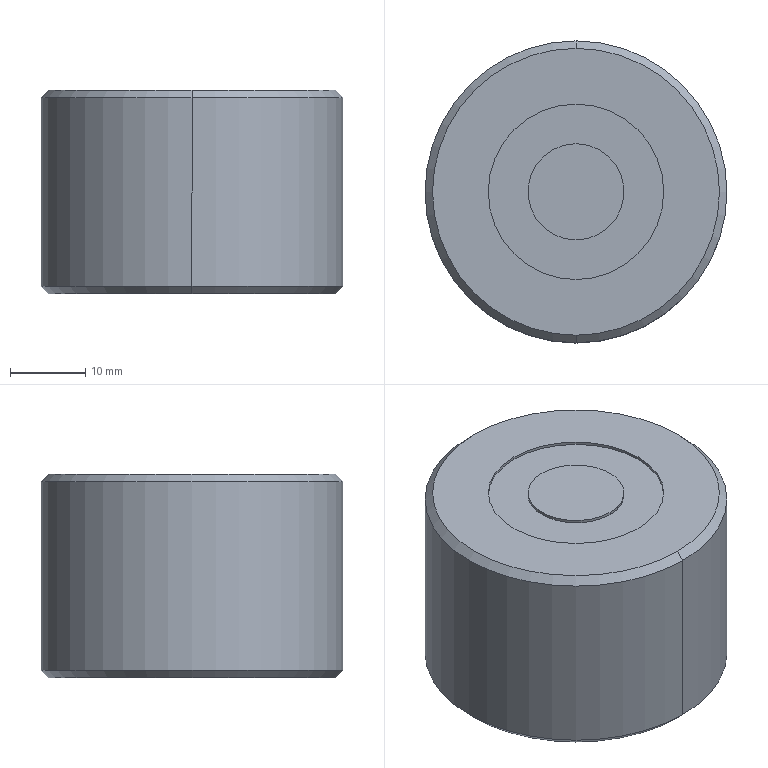Part | SolidWorks | features BaseBody 1 | 1 solid | 22 faces | box 40 x 40 x 27 mm | volume 33590 mm3 | cone 10 | cylinder 8 | plane 4 | commonest cylinder face diameters 3.3 x2 12.741 x2 23.241 x2 40 x2
STEP:
#1=CARTESIAN_POINT('',(489.266,-74.349,254.748));
#2=VERTEX_POINT('',#1);
#3=CARTESIAN_POINT('',(489.266,-34.349,254.748));
#4=VERTEX_POINT('',#3);
#5=CARTESIAN_POINT('',(489.266,-54.349,254.748));
#6=DIRECTION('',(0.000000004,-0.000000009,1.));
#7=DIRECTION('',(0.,-1.,-0.000000009));
#8=AXIS2_PLACEMENT_3D('',#5,#6,#7);
#9=CIRCLE('',#8,20.);
#10=EDGE_CURVE('',#2,#4,#9,.T.);
#11=ORIENTED_EDGE('',*,*,#10,.T.);
#12=CARTESIAN_POINT('',(489.266,-34.349,279.748));
#13=VERTEX_POINT('',#12);
#14=CARTESIAN_POINT('',(489.266,-34.349,280.748));
#15=DIRECTION('',(0.000000004,-0.000000009,1.));
#16=VECTOR('',#15,1000.);
#17=LINE('',#14,#16);
#18=EDGE_CURVE('',#4,#13,#17,.T.);
#19=ORIENTED_EDGE('',*,*,#18,.T.);
#20=CARTESIAN_POINT('',(489.266,-74.349,279.748));
#21=VERTEX_POINT('',#20);
#22=CARTESIAN_POINT('',(489.266,-54.349,279.748));
#23=DIRECTION('',(-0.000000004,0.000000009,-1.));
#24=DIRECTION('',(0.,-1.,-0.000000009));
#25=AXIS2_PLACEMENT_3D('',#22,#23,#24);
#26=CIRCLE('',#25,20.);
#27=EDGE_CURVE('',#13,#21,#26,.T.);
#28=ORIENTED_EDGE('',*,*,#27,.T.);
#29=CARTESIAN_POINT('',(489.266,-74.349,280.748));
#30=DIRECTION('',(0.000000004,-0.000000009,1.));
#31=VECTOR('',#30,1000.);
#32=LINE('',#29,#31);
#33=EDGE_CURVE('',#2,#21,#32,.T.);
#34=ORIENTED_EDGE('',*,*,#33,.F.);
#35=EDGE_LOOP('',(#11,#19,#28,#34));
#36=FACE_OUTER_BOUND('',#35,.T.);
#37=CARTESIAN_POINT('',(489.266,-54.349,280.748));
#38=DIRECTION('',(0.000000004,-0.000000009,1.));
#39=DIRECTION('',(0.,-1.,-0.000000009));
#40=AXIS2_PLACEMENT_3D('',#37,#38,#39);
#41=CYLINDRICAL_SURFACE('',#40,20.);
#42=ADVANCED_FACE('',(#36),#41,.T.);
#43=CARTESIAN_POINT('',(489.266,-35.349,280.748));
#44=VERTEX_POINT('',#43);
#45=CARTESIAN_POINT('',(489.266,-73.349,280.748));
#46=VERTEX_POINT('',#45);
#47=CARTESIAN_POINT('',(489.266,-54.349,280.748));
#48=DIRECTION('',(-0.000000004,0.000000009,-1.));
#49=DIRECTION('',(0.,1.,0.000000009));
#50=AXIS2_PLACEMENT_3D('',#47,#48,#49);
#51=CIRCLE('',#50,19.);
#52=EDGE_CURVE('',#44,#46,#51,.T.);
#53=ORIENTED_EDGE('',*,*,#52,.T.);
#54=CARTESIAN_POINT('',(489.266,-74.349,279.748));
#55=DIRECTION('',(-0.000000003,-0.7071,-0.7071));
#56=VECTOR('',#55,1000.);
#57=LINE('',#54,#56);
#58=EDGE_CURVE('',#46,#21,#57,.T.);
#59=ORIENTED_EDGE('',*,*,#58,.T.);
#60=ORIENTED_EDGE('',*,*,#27,.F.);
#61=CARTESIAN_POINT('',(489.266,-34.349,279.748));
#62=DIRECTION('',(-0.000000003,0.7071,-0.7071));
#63=VECTOR('',#62,1000.);
#64=LINE('',#61,#63);
#65=EDGE_CURVE('',#44,#13,#64,.T.);
#66=ORIENTED_EDGE('',*,*,#65,.F.);
#67=EDGE_LOOP('',(#53,#59,#60,#66));
#68=FACE_OUTER_BOUND('',#67,.T.);
#69=CARTESIAN_POINT('',(489.266,-54.349,279.748));
#70=DIRECTION('',(-0.000000004,0.000000009,-1.));
#71=DIRECTION('',(0.,1.,0.000000009));
#72=AXIS2_PLACEMENT_3D('',#69,#70,#71);
#73=CONICAL_SURFACE('',#72,20.,0.7854);
#74=ADVANCED_FACE('',(#68),#73,.T.);
#75=CARTESIAN_POINT('',(489.266,-73.349,253.748));
#76=VERTEX_POINT('',#75);
#77=CARTESIAN_POINT('',(489.266,-35.349,253.748));
#78=VERTEX_POINT('',#77);
#79=CARTESIAN_POINT('',(489.266,-54.349,253.748));
#80=DIRECTION('',(0.000000004,-0.000000009,1.));
#81=DIRECTION('',(0.,-1.,-0.000000009));
#82=AXIS2_PLACEMENT_3D('',#79,#80,#81);
#83=CIRCLE('',#82,19.);
#84=EDGE_CURVE('',#76,#78,#83,.T.);
#85=ORIENTED_EDGE('',*,*,#84,.T.);
#86=CARTESIAN_POINT('',(489.266,-34.349,254.748));
#87=DIRECTION('',(0.000000003,0.7071,0.7071));
#88=VECTOR('',#87,1000.);
#89=LINE('',#86,#88);
#90=EDGE_CURVE('',#78,#4,#89,.T.);
#91=ORIENTED_EDGE('',*,*,#90,.T.);
#92=ORIENTED_EDGE('',*,*,#10,.F.);
#93=CARTESIAN_POINT('',(489.266,-74.349,254.748));
#94=DIRECTION('',(0.000000003,-0.7071,0.7071));
#95=VECTOR('',#94,1000.);
#96=LINE('',#93,#95);
#97=EDGE_CURVE('',#76,#2,#96,.T.);
#98=ORIENTED_EDGE('',*,*,#97,.F.);
#99=EDGE_LOOP('',(#85,#91,#92,#98));
#100=FACE_OUTER_BOUND('',#99,.T.);
#101=CARTESIAN_POINT('',(489.266,-54.349,254.748));
#102=DIRECTION('',(0.000000004,-0.000000009,1.));
#103=DIRECTION('',(0.,-1.,-0.000000009));
#104=AXIS2_PLACEMENT_3D('',#101,#102,#103);
#105=CONICAL_SURFACE('',#104,20.,0.7854);
#106=ADVANCED_FACE('',(#100),#105,.T.);
#107=CARTESIAN_POINT('',(489.266,-42.729,280.377));
#108=VERTEX_POINT('',#107);
#109=CARTESIAN_POINT('',(489.266,-65.969,280.377));
#110=VERTEX_POINT('',#109);
#111=CARTESIAN_POINT('',(489.266,-54.349,280.377));
#112=DIRECTION('',(0.000000004,-0.000000009,1.));
#113=DIRECTION('',(0.,-1.,-0.000000009));
#114=AXIS2_PLACEMENT_3D('',#111,#112,#113);
#115=CIRCLE('',#114,11.62);
#116=EDGE_CURVE('',#108,#110,#115,.T.);
#117=ORIENTED_EDGE('',*,*,#116,.F.);
#118=CARTESIAN_POINT('',(489.266,-42.729,280.748));
#119=VERTEX_POINT('',#118);
#120=CARTESIAN_POINT('',(489.266,-42.729,281.353));
#121=DIRECTION('',(0.000000004,-0.000000009,1.));
#122=VECTOR('',#121,1000.);
#123=LINE('',#120,#122);
#124=EDGE_CURVE('',#108,#119,#123,.T.);
#125=ORIENTED_EDGE('',*,*,#124,.T.);
#126=CARTESIAN_POINT('',(489.266,-65.969,280.748));
#127=VERTEX_POINT('',#126);
#128=CARTESIAN_POINT('',(489.266,-54.349,280.748));
#129=DIRECTION('',(0.000000004,-0.000000009,1.));
#130=DIRECTION('',(0.,-1.,-0.000000009));
#131=AXIS2_PLACEMENT_3D('',#128,#129,#130);
#132=CIRCLE('',#131,11.62);
#133=EDGE_CURVE('',#119,#127,#132,.T.);
#134=ORIENTED_EDGE('',*,*,#133,.T.);
#135=CARTESIAN_POINT('',(489.266,-65.969,281.353));
#136=DIRECTION('',(0.000000004,-0.000000009,1.));
#137=VECTOR('',#136,1000.);
#138=LINE('',#135,#137);
#139=EDGE_CURVE('',#110,#127,#138,.T.);
#140=ORIENTED_EDGE('',*,*,#139,.F.);
#141=EDGE_LOOP('',(#117,#125,#134,#140));
#142=FACE_OUTER_BOUND('',#141,.T.);
#143=CARTESIAN_POINT('',(489.266,-54.349,281.353));
#144=DIRECTION('',(0.000000004,-0.000000009,1.));
#145=DIRECTION('',(0.,-1.,-0.000000009));
#146=AXIS2_PLACEMENT_3D('',#143,#144,#145);
#147=CYLINDRICAL_SURFACE('',#146,11.62);
#148=ADVANCED_FACE('',(#142),#147,.F.);
#149=CARTESIAN_POINT('',(489.266,-55.999,254.048));
#150=VERTEX_POINT('',#149);
#151=CARTESIAN_POINT('',(489.266,-52.699,254.048));
#152=VERTEX_POINT('',#151);
#153=CARTESIAN_POINT('',(489.266,-54.349,254.048));
#154=DIRECTION('',(-0.000000004,0.000000009,-1.));
#155=DIRECTION('',(0.5198,-0.8543,-0.000000009));
#156=AXIS2_PLACEMENT_3D('',#153,#154,#155);
#157=CIRCLE('',#156,1.65);
#158=EDGE_CURVE('',#150,#152,#157,.T.);
#159=ORIENTED_EDGE('',*,*,#158,.F.);
#160=CARTESIAN_POINT('',(489.266,-56.299,253.748));
#161=VERTEX_POINT('',#160);
#162=CARTESIAN_POINT('',(489.266,-56.299,253.748));
#163=DIRECTION('',(-0.000000003,-0.7071,-0.7071));
#164=VECTOR('',#163,1000.);
#165=LINE('',#162,#164);
#166=EDGE_CURVE('',#150,#161,#165,.T.);
#167=ORIENTED_EDGE('',*,*,#166,.T.);
#168=CARTESIAN_POINT('',(489.266,-52.399,253.748));
#169=VERTEX_POINT('',#168);
#170=CARTESIAN_POINT('',(489.266,-54.349,253.748));
#171=DIRECTION('',(0.000000004,-0.000000009,1.));
#172=DIRECTION('',(0.,1.,0.000000009));
#173=AXIS2_PLACEMENT_3D('',#170,#171,#172);
#174=CIRCLE('',#173,1.95);
#175=EDGE_CURVE('',#169,#161,#174,.T.);
#176=ORIENTED_EDGE('',*,*,#175,.F.);
#177=CARTESIAN_POINT('',(489.266,-52.399,253.748));
#178=DIRECTION('',(-0.000000003,0.7071,-0.7071));
#179=VECTOR('',#178,1000.);
#180=LINE('',#177,#179);
#181=EDGE_CURVE('',#152,#169,#180,.T.);
#182=ORIENTED_EDGE('',*,*,#181,.F.);
#183=EDGE_LOOP('',(#159,#167,#176,#182));
#184=FACE_OUTER_BOUND('',#183,.T.);
#185=CARTESIAN_POINT('',(489.266,-54.349,253.748));
#186=DIRECTION('',(-0.000000004,0.000000009,-1.));
#187=DIRECTION('',(0.,1.,0.000000009));
#188=AXIS2_PLACEMENT_3D('',#185,#186,#187);
#189=CONICAL_SURFACE('',#188,1.95,0.7854);
#190=ADVANCED_FACE('',(#184),#189,.F.);
#191=ORIENTED_EDGE('',*,*,#158,.T.);
#192=CARTESIAN_POINT('',(489.266,-52.699,263.748));
#193=VERTEX_POINT('',#192);
#194=CARTESIAN_POINT('',(489.266,-52.699,258.748));
#195=DIRECTION('',(0.000000004,-0.000000009,1.));
#196=VECTOR('',#195,1000.);
#197=LINE('',#194,#196);
#198=EDGE_CURVE('',#152,#193,#197,.T.);
#199=ORIENTED_EDGE('',*,*,#198,.T.);
#200=CARTESIAN_POINT('',(489.266,-55.999,263.748));
#201=VERTEX_POINT('',#200);
#202=CARTESIAN_POINT('',(489.266,-54.349,263.748));
#203=DIRECTION('',(-0.000000004,0.000000009,-1.));
#204=DIRECTION('',(0.,-1.,-0.000000009));
#205=AXIS2_PLACEMENT_3D('',#202,#203,#204);
#206=CIRCLE('',#205,1.65);
#207=EDGE_CURVE('',#201,#193,#206,.T.);
#208=ORIENTED_EDGE('',*,*,#207,.F.);
#209=CARTESIAN_POINT('',(489.266,-55.999,258.748));
#210=DIRECTION('',(0.000000004,-0.000000009,1.));
#211=VECTOR('',#210,1000.);
#212=LINE('',#209,#211);
#213=EDGE_CURVE('',#150,#201,#212,.T.);
#214=ORIENTED_EDGE('',*,*,#213,.F.);
#215=EDGE_LOOP('',(#191,#199,#208,#214));
#216=FACE_OUTER_BOUND('',#215,.T.);
#217=CARTESIAN_POINT('',(489.266,-54.349,258.748));
#218=DIRECTION('',(0.000000004,-0.000000009,1.));
#219=DIRECTION('',(0.,-1.,-0.000000009));
#220=AXIS2_PLACEMENT_3D('',#217,#218,#219);
#221=CYLINDRICAL_SURFACE('',#220,1.65);
#222=ADVANCED_FACE('',(#216),#221,.F.);
#223=CARTESIAN_POINT('',(489.266,-47.979,280.748));
#224=VERTEX_POINT('',#223);
#225=CARTESIAN_POINT('',(489.266,-60.72,280.748));
#226=VERTEX_POINT('',#225);
#227=CARTESIAN_POINT('',(489.266,-54.349,280.748));
#228=DIRECTION('',(-0.000000004,0.000000009,-1.));
#229=DIRECTION('',(0.,1.,0.000000009));
#230=AXIS2_PLACEMENT_3D('',#227,#228,#229);
#231=CIRCLE('',#230,6.37);
#232=EDGE_CURVE('',#224,#226,#231,.T.);
#233=ORIENTED_EDGE('',*,*,#232,.T.);
#234=CARTESIAN_POINT('',(489.266,-60.72,280.377));
#235=VERTEX_POINT('',#234);
#236=CARTESIAN_POINT('',(489.266,-60.72,280.377));
#237=DIRECTION('',(-0.000000004,0.000000009,-1.));
#238=VECTOR('',#237,1000.);
#239=LINE('',#236,#238);
#240=EDGE_CURVE('',#226,#235,#239,.T.);
#241=ORIENTED_EDGE('',*,*,#240,.T.);
#242=CARTESIAN_POINT('',(489.266,-47.979,280.377));
#243=VERTEX_POINT('',#242);
#244=CARTESIAN_POINT('',(489.266,-54.349,280.377));
#245=DIRECTION('',(0.000000004,-0.000000009,1.));
#246=DIRECTION('',(0.,1.,0.000000009));
#247=AXIS2_PLACEMENT_3D('',#244,#245,#246);
#248=CIRCLE('',#247,6.37);
#249=EDGE_CURVE('',#235,#243,#248,.T.);
#250=ORIENTED_EDGE('',*,*,#249,.T.);
#251=CARTESIAN_POINT('',(489.266,-47.979,280.377));
#252=DIRECTION('',(-0.000000004,0.000000009,-1.));
#253=VECTOR('',#252,1000.);
#254=LINE('',#251,#253);
#255=EDGE_CURVE('',#224,#243,#254,.T.);
#256=ORIENTED_EDGE('',*,*,#255,.F.);
#257=EDGE_LOOP('',(#233,#241,#250,#256));
#258=FACE_OUTER_BOUND('',#257,.T.);
#259=CARTESIAN_POINT('',(489.266,-54.349,280.377));
#260=DIRECTION('',(-0.000000004,0.000000009,-1.));
#261=DIRECTION('',(0.,1.,0.000000009));
#262=AXIS2_PLACEMENT_3D('',#259,#260,#261);
#263=CYLINDRICAL_SURFACE('',#262,6.37);
#264=ADVANCED_FACE('',(#258),#263,.T.);
#265=CARTESIAN_POINT('',(489.266,-55.999,265.748));
#266=VERTEX_POINT('',#265);
#267=CARTESIAN_POINT('',(489.266,-52.699,265.748));
#268=VERTEX_POINT('',#267);
#269=CARTESIAN_POINT('',(489.266,-54.349,265.748));
#270=DIRECTION('',(-0.000000004,0.000000009,-1.));
#271=DIRECTION('',(0.,1.,0.000000009));
#272=AXIS2_PLACEMENT_3D('',#269,#270,#271);
#273=CIRCLE('',#272,1.65);
#274=EDGE_CURVE('',#266,#268,#273,.T.);
#275=ORIENTED_EDGE('',*,*,#274,.F.);
#276=CARTESIAN_POINT('',(489.266,-55.999,263.748));
#277=DIRECTION('',(-0.000000004,-0.000008241,-1.));
#278=VECTOR('',#277,1000.);
#279=LINE('',#276,#278);
#280=EDGE_CURVE('',#266,#201,#279,.T.);
#281=ORIENTED_EDGE('',*,*,#280,.T.);
#282=ORIENTED_EDGE('',*,*,#207,.T.);
#283=CARTESIAN_POINT('',(489.266,-52.699,263.748));
#284=DIRECTION('',(-0.000000004,0.000008259,-1.));
#285=VECTOR('',#284,1000.);
#286=LINE('',#283,#285);
#287=EDGE_CURVE('',#268,#193,#286,.T.);
#288=ORIENTED_EDGE('',*,*,#287,.F.);
#289=EDGE_LOOP('',(#275,#281,#282,#288));
#290=FACE_OUTER_BOUND('',#289,.T.);
#291=CARTESIAN_POINT('',(489.266,-54.349,263.748));
#292=DIRECTION('',(-0.000000004,0.000000009,-1.));
#293=DIRECTION('',(0.,1.,0.000000009));
#294=AXIS2_PLACEMENT_3D('',#291,#292,#293);
#295=CONICAL_SURFACE('',#294,1.65,0.00000825);
#296=ADVANCED_FACE('',(#290),#295,.F.);
#297=CARTESIAN_POINT('',(489.266,-54.349,266.739));
#298=VERTEX_POINT('',#297);
#299=CARTESIAN_POINT('',(489.266,-52.699,265.748));
#300=DIRECTION('',(-0.000000002,0.8572,-0.515));
#301=VECTOR('',#300,1000.);
#302=LINE('',#299,#301);
#303=EDGE_CURVE('',#298,#268,#302,.T.);
#304=ORIENTED_EDGE('',*,*,#303,.F.);
#305=CARTESIAN_POINT('',(489.266,-55.999,265.748));
#306=DIRECTION('',(-0.000000002,-0.8572,-0.515));
#307=VECTOR('',#306,1000.);
#308=LINE('',#305,#307);
#309=EDGE_CURVE('',#298,#266,#308,.T.);
#310=ORIENTED_EDGE('',*,*,#309,.T.);
#311=ORIENTED_EDGE('',*,*,#274,.T.);
#312=EDGE_LOOP('',(#304,#310,#311));
#313=FACE_OUTER_BOUND('',#312,.T.);
#314=CARTESIAN_POINT('',(489.266,-54.349,265.748));
#315=DIRECTION('',(-0.000000004,0.000000009,-1.));
#316=DIRECTION('',(0.,1.,0.000000009));
#317=AXIS2_PLACEMENT_3D('',#314,#315,#316);
#318=CONICAL_SURFACE('',#317,1.65,1.03);
#319=ADVANCED_FACE('',(#313),#318,.F.);
#320=ORIENTED_EDGE('',*,*,#18,.F.);
#321=CARTESIAN_POINT('',(489.266,-54.349,254.748));
#322=DIRECTION('',(0.000000004,-0.000000009,1.));
#323=DIRECTION('',(0.,-1.,-0.000000009));
#324=AXIS2_PLACEMENT_3D('',#321,#322,#323);
#325=CIRCLE('',#324,20.);
#326=EDGE_CURVE('',#4,#2,#325,.T.);
#327=ORIENTED_EDGE('',*,*,#326,.T.);
#328=ORIENTED_EDGE('',*,*,#33,.T.);
#329=CARTESIAN_POINT('',(489.266,-54.349,279.748));
#330=DIRECTION('',(-0.000000004,0.000000009,-1.));
#331=DIRECTION('',(0.,-1.,-0.000000009));
#332=AXIS2_PLACEMENT_3D('',#329,#330,#331);
#333=CIRCLE('',#332,20.);
#334=EDGE_CURVE('',#21,#13,#333,.T.);
#335=ORIENTED_EDGE('',*,*,#334,.T.);
#336=EDGE_LOOP('',(#320,#327,#328,#335));
#337=FACE_OUTER_BOUND('',#336,.T.);
#338=CARTESIAN_POINT('',(489.266,-54.349,280.748));
#339=DIRECTION('',(0.000000004,-0.000000009,1.));
#340=DIRECTION('',(0.,-1.,-0.000000009));
#341=AXIS2_PLACEMENT_3D('',#338,#339,#340);
#342=CYLINDRICAL_SURFACE('',#341,20.);
#343=ADVANCED_FACE('',(#337),#342,.T.);
#344=ORIENTED_EDGE('',*,*,#58,.F.);
#345=CARTESIAN_POINT('',(489.266,-54.349,280.748));
#346=DIRECTION('',(-0.000000004,0.000000009,-1.));
#347=DIRECTION('',(0.,1.,0.000000009));
#348=AXIS2_PLACEMENT_3D('',#345,#346,#347);
#349=CIRCLE('',#348,19.);
#350=EDGE_CURVE('',#46,#44,#349,.T.);
#351=ORIENTED_EDGE('',*,*,#350,.T.);
#352=ORIENTED_EDGE('',*,*,#65,.T.);
#353=ORIENTED_EDGE('',*,*,#334,.F.);
#354=EDGE_LOOP('',(#344,#351,#352,#353));
#355=FACE_OUTER_BOUND('',#354,.T.);
#356=CARTESIAN_POINT('',(489.266,-54.349,279.748));
#357=DIRECTION('',(-0.000000004,0.000000009,-1.));
#358=DIRECTION('',(0.,1.,0.000000009));
#359=AXIS2_PLACEMENT_3D('',#356,#357,#358);
#360=CONICAL_SURFACE('',#359,20.,0.7854);
#361=ADVANCED_FACE('',(#355),#360,.T.);
#362=ORIENTED_EDGE('',*,*,#90,.F.);
#363=CARTESIAN_POINT('',(489.266,-54.349,253.748));
#364=DIRECTION('',(0.000000004,-0.000000009,1.));
#365=DIRECTION('',(0.,-1.,-0.000000009));
#366=AXIS2_PLACEMENT_3D('',#363,#364,#365);
#367=CIRCLE('',#366,19.);
#368=EDGE_CURVE('',#78,#76,#367,.T.);
#369=ORIENTED_EDGE('',*,*,#368,.T.);
#370=ORIENTED_EDGE('',*,*,#97,.T.);
#371=ORIENTED_EDGE('',*,*,#326,.F.);
#372=EDGE_LOOP('',(#362,#369,#370,#371));
#373=FACE_OUTER_BOUND('',#372,.T.);
#374=CARTESIAN_POINT('',(489.266,-54.349,254.748));
#375=DIRECTION('',(0.000000004,-0.000000009,1.));
#376=DIRECTION('',(0.,-1.,-0.000000009));
#377=AXIS2_PLACEMENT_3D('',#374,#375,#376);
#378=CONICAL_SURFACE('',#377,20.,0.7854);
#379=ADVANCED_FACE('',(#373),#378,.T.);
#380=ORIENTED_EDGE('',*,*,#52,.F.);
#381=ORIENTED_EDGE('',*,*,#350,.F.);
#382=EDGE_LOOP('',(#380,#381));
#383=FACE_OUTER_BOUND('',#382,.T.);
#384=CARTESIAN_POINT('',(489.266,-54.349,280.748));
#385=DIRECTION('',(0.000000004,-0.000000009,1.));
#386=DIRECTION('',(0.,-1.,-0.000000009));
#387=AXIS2_PLACEMENT_3D('',#384,#385,#386);
#388=CIRCLE('',#387,11.62);
#389=EDGE_CURVE('',#127,#119,#388,.T.);
#390=ORIENTED_EDGE('',*,*,#389,.F.);
#391=ORIENTED_EDGE('',*,*,#133,.F.);
#392=EDGE_LOOP('',(#390,#391));
#393=FACE_BOUND('',#392,.T.);
#394=CARTESIAN_POINT('',(489.266,-54.349,280.748));
#395=DIRECTION('',(-0.000000004,0.000000009,-1.));
#396=DIRECTION('',(0.,1.,0.000000009));
#397=AXIS2_PLACEMENT_3D('',#394,#395,#396);
#398=PLANE('',#397);
#399=ADVANCED_FACE('',(#383,#393),#398,.F.);
#400=ORIENTED_EDGE('',*,*,#175,.T.);
#401=CARTESIAN_POINT('',(489.266,-54.349,253.748));
#402=DIRECTION('',(0.000000004,-0.000000009,1.));
#403=DIRECTION('',(0.,1.,0.000000009));
#404=AXIS2_PLACEMENT_3D('',#401,#402,#403);
#405=CIRCLE('',#404,1.95);
#406=EDGE_CURVE('',#161,#169,#405,.T.);
#407=ORIENTED_EDGE('',*,*,#406,.T.);
#408=EDGE_LOOP('',(#400,#407));
#409=FACE_BOUND('',#408,.T.);
#410=ORIENTED_EDGE('',*,*,#84,.F.);
#411=ORIENTED_EDGE('',*,*,#368,.F.);
#412=EDGE_LOOP('',(#410,#411));
#413=FACE_OUTER_BOUND('',#412,.T.);
#414=CARTESIAN_POINT('',(489.266,-54.349,253.748));
#415=DIRECTION('',(-0.000000004,0.000000009,-1.));
#416=DIRECTION('',(0.,1.,0.000000009));
#417=AXIS2_PLACEMENT_3D('',#414,#415,#416);
#418=PLANE('',#417);
#419=ADVANCED_FACE('',(#409,#413),#418,.T.);
#420=ORIENTED_EDGE('',*,*,#124,.F.);
#421=CARTESIAN_POINT('',(489.266,-54.349,280.377));
#422=DIRECTION('',(0.000000004,-0.000000009,1.));
#423=DIRECTION('',(0.,-1.,-0.000000009));
#424=AXIS2_PLACEMENT_3D('',#421,#422,#423);
#425=CIRCLE('',#424,11.62);
#426=EDGE_CURVE('',#110,#108,#425,.T.);
#427=ORIENTED_EDGE('',*,*,#426,.F.);
#428=ORIENTED_EDGE('',*,*,#139,.T.);
#429=ORIENTED_EDGE('',*,*,#389,.T.);
#430=EDGE_LOOP('',(#420,#427,#428,#429));
#431=FACE_OUTER_BOUND('',#430,.T.);
#432=CARTESIAN_POINT('',(489.266,-54.349,281.353));
#433=DIRECTION('',(0.000000004,-0.000000009,1.));
#434=DIRECTION('',(0.,-1.,-0.000000009));
#435=AXIS2_PLACEMENT_3D('',#432,#433,#434);
#436=CYLINDRICAL_SURFACE('',#435,11.62);
#437=ADVANCED_FACE('',(#431),#436,.F.);
#438=ORIENTED_EDGE('',*,*,#166,.F.);
#439=CARTESIAN_POINT('',(489.266,-54.349,254.048));
#440=DIRECTION('',(-0.000000004,0.000000009,-1.));
#441=DIRECTION('',(0.5198,-0.8543,-0.000000009));
#442=AXIS2_PLACEMENT_3D('',#439,#440,#441);
#443=CIRCLE('',#442,1.65);
#444=EDGE_CURVE('',#152,#150,#443,.T.);
#445=ORIENTED_EDGE('',*,*,#444,.F.);
#446=ORIENTED_EDGE('',*,*,#181,.T.);
#447=ORIENTED_EDGE('',*,*,#406,.F.);
#448=EDGE_LOOP('',(#438,#445,#446,#447));
#449=FACE_OUTER_BOUND('',#448,.T.);
#450=CARTESIAN_POINT('',(489.266,-54.349,253.748));
#451=DIRECTION('',(-0.000000004,0.000000009,-1.));
#452=DIRECTION('',(0.,1.,0.000000009));
#453=AXIS2_PLACEMENT_3D('',#450,#451,#452);
#454=CONICAL_SURFACE('',#453,1.95,0.7854);
#455=ADVANCED_FACE('',(#449),#454,.F.);
#456=ORIENTED_EDGE('',*,*,#426,.T.);
#457=ORIENTED_EDGE('',*,*,#116,.T.);
#458=EDGE_LOOP('',(#456,#457));
#459=FACE_OUTER_BOUND('',#458,.T.);
#460=CARTESIAN_POINT('',(489.266,-54.349,280.377));
#461=DIRECTION('',(0.000000004,-0.000000009,1.));
#462=DIRECTION('',(0.,1.,0.000000009));
#463=AXIS2_PLACEMENT_3D('',#460,#461,#462);
#464=CIRCLE('',#463,6.37);
#465=EDGE_CURVE('',#243,#235,#464,.T.);
#466=ORIENTED_EDGE('',*,*,#465,.F.);
#467=ORIENTED_EDGE('',*,*,#249,.F.);
#468=EDGE_LOOP('',(#466,#467));
#469=FACE_BOUND('',#468,.T.);
#470=CARTESIAN_POINT('',(489.266,-54.349,280.377));
#471=DIRECTION('',(-0.000000004,0.000000009,-1.));
#472=DIRECTION('',(0.,1.,0.000000009));
#473=AXIS2_PLACEMENT_3D('',#470,#471,#472);
#474=PLANE('',#473);
#475=ADVANCED_FACE('',(#459,#469),#474,.F.);
#476=ORIENTED_EDGE('',*,*,#198,.F.);
#477=ORIENTED_EDGE('',*,*,#444,.T.);
#478=ORIENTED_EDGE('',*,*,#213,.T.);
#479=CARTESIAN_POINT('',(489.266,-54.349,263.748));
#480=DIRECTION('',(-0.000000004,0.000000009,-1.));
#481=DIRECTION('',(0.,-1.,-0.000000009));
#482=AXIS2_PLACEMENT_3D('',#479,#480,#481);
#483=CIRCLE('',#482,1.65);
#484=EDGE_CURVE('',#193,#201,#483,.T.);
#485=ORIENTED_EDGE('',*,*,#484,.F.);
#486=EDGE_LOOP('',(#476,#477,#478,#485));
#487=FACE_OUTER_BOUND('',#486,.T.);
#488=CARTESIAN_POINT('',(489.266,-54.349,258.748));
#489=DIRECTION('',(0.000000004,-0.000000009,1.));
#490=DIRECTION('',(0.,-1.,-0.000000009));
#491=AXIS2_PLACEMENT_3D('',#488,#489,#490);
#492=CYLINDRICAL_SURFACE('',#491,1.65);
#493=ADVANCED_FACE('',(#487),#492,.F.);
#494=ORIENTED_EDGE('',*,*,#240,.F.);
#495=CARTESIAN_POINT('',(489.266,-54.349,280.748));
#496=DIRECTION('',(-0.000000004,0.000000009,-1.));
#497=DIRECTION('',(0.,1.,0.000000009));
#498=AXIS2_PLACEMENT_3D('',#495,#496,#497);
#499=CIRCLE('',#498,6.37);
#500=EDGE_CURVE('',#226,#224,#499,.T.);
#501=ORIENTED_EDGE('',*,*,#500,.T.);
#502=ORIENTED_EDGE('',*,*,#255,.T.);
#503=ORIENTED_EDGE('',*,*,#465,.T.);
#504=EDGE_LOOP('',(#494,#501,#502,#503));
#505=FACE_OUTER_BOUND('',#504,.T.);
#506=CARTESIAN_POINT('',(489.266,-54.349,280.377));
#507=DIRECTION('',(-0.000000004,0.000000009,-1.));
#508=DIRECTION('',(0.,1.,0.000000009));
#509=AXIS2_PLACEMENT_3D('',#506,#507,#508);
#510=CYLINDRICAL_SURFACE('',#509,6.37);
#511=ADVANCED_FACE('',(#505),#510,.T.);
#512=ORIENTED_EDGE('',*,*,#280,.F.);
#513=CARTESIAN_POINT('',(489.266,-54.349,265.748));
#514=DIRECTION('',(-0.000000004,0.000000009,-1.));
#515=DIRECTION('',(0.,1.,0.000000009));
#516=AXIS2_PLACEMENT_3D('',#513,#514,#515);
#517=CIRCLE('',#516,1.65);
#518=EDGE_CURVE('',#268,#266,#517,.T.);
#519=ORIENTED_EDGE('',*,*,#518,.F.);
#520=ORIENTED_EDGE('',*,*,#287,.T.);
#521=ORIENTED_EDGE('',*,*,#484,.T.);
#522=EDGE_LOOP('',(#512,#519,#520,#521));
#523=FACE_OUTER_BOUND('',#522,.T.);
#524=CARTESIAN_POINT('',(489.266,-54.349,263.748));
#525=DIRECTION('',(-0.000000004,0.000000009,-1.));
#526=DIRECTION('',(0.,1.,0.000000009));
#527=AXIS2_PLACEMENT_3D('',#524,#525,#526);
#528=CONICAL_SURFACE('',#527,1.65,0.00000825);
#529=ADVANCED_FACE('',(#523),#528,.F.);
#530=ORIENTED_EDGE('',*,*,#232,.F.);
#531=ORIENTED_EDGE('',*,*,#500,.F.);
#532=EDGE_LOOP('',(#530,#531));
#533=FACE_OUTER_BOUND('',#532,.T.);
#534=CARTESIAN_POINT('',(489.266,-54.349,280.748));
#535=DIRECTION('',(0.000000004,-0.000000009,1.));
#536=DIRECTION('',(0.,-1.,-0.000000009));
#537=AXIS2_PLACEMENT_3D('',#534,#535,#536);
#538=PLANE('',#537);
#539=ADVANCED_FACE('',(#533),#538,.T.);
#540=ORIENTED_EDGE('',*,*,#309,.F.);
#541=ORIENTED_EDGE('',*,*,#303,.T.);
#542=ORIENTED_EDGE('',*,*,#518,.T.);
#543=EDGE_LOOP('',(#540,#541,#542));
#544=FACE_OUTER_BOUND('',#543,.T.);
#545=CARTESIAN_POINT('',(489.266,-54.349,265.748));
#546=DIRECTION('',(-0.000000004,0.000000009,-1.));
#547=DIRECTION('',(0.,1.,0.000000009));
#548=AXIS2_PLACEMENT_3D('',#545,#546,#547);
#549=CONICAL_SURFACE('',#548,1.65,1.03);
#550=ADVANCED_FACE('',(#544),#549,.F.);
#551=CLOSED_SHELL('',(#42,#74,#106,#148,#190,#222,#264,#296,#319,#343,#361,#379,#399,#419,#437,#455,#475,#493,#511,#529,#539,#550));
#552=MANIFOLD_SOLID_BREP('',#551);
#553=CARTESIAN_POINT('',(0.,0.,0.));
#554=DIRECTION('',(0.,0.,1.));
#555=DIRECTION('',(1.,0.,0.));
#556=AXIS2_PLACEMENT_3D('',#553,#554,#555);
#557=(LENGTH_UNIT()NAMED_UNIT(*)SI_UNIT(.MILLI.,.METRE.));
#558=UNCERTAINTY_MEASURE_WITH_UNIT(LENGTH_MEASURE(0.00001),#557,'','');
#559=(NAMED_UNIT(*)PLANE_ANGLE_UNIT()SI_UNIT($,.RADIAN.));
#560=(NAMED_UNIT(*)SI_UNIT($,.STERADIAN.)SOLID_ANGLE_UNIT());
#561=(GEOMETRIC_REPRESENTATION_CONTEXT(3)GLOBAL_UNCERTAINTY_ASSIGNED_CONTEXT((#558))GLOBAL_UNIT_ASSIGNED_CONTEXT((#557,#559,#560))REPRESENTATION_CONTEXT('',''));
#562=ADVANCED_BREP_SHAPE_REPRESENTATION('',(#552,#556),#561);